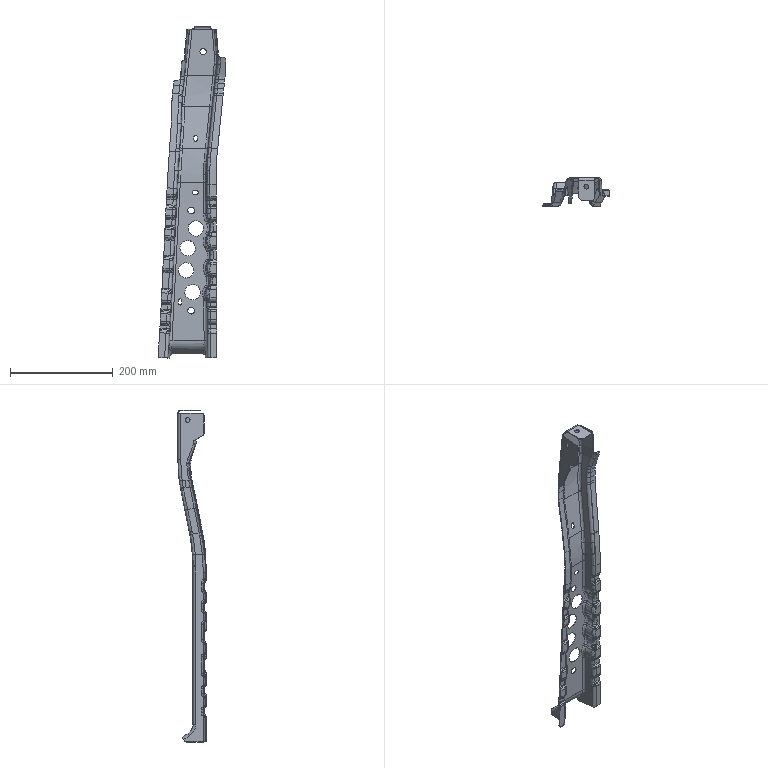Part | 1 solid | 867 faces | box 131.065 x 55.209 x 645.962 mm | volume 103415 mm3 | spline 376 | cylinder 288 | plane 137 | sphere 48 | other 18 | commonest cylinder face diameters 10 x98 12.4 x75 7.6 x22 12 x20 9.6 x18 30 x9